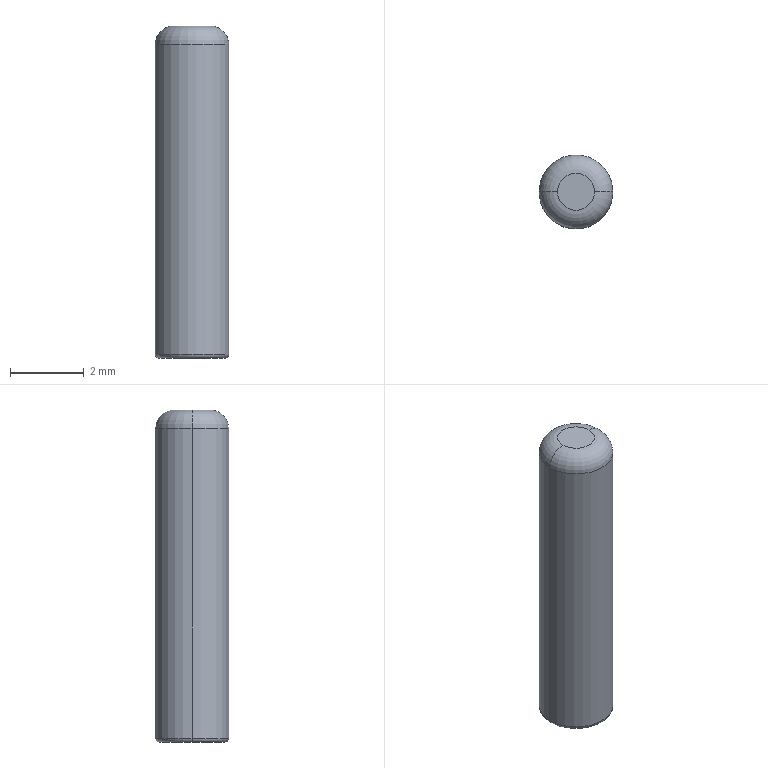Part | SolidWorks | features Fillet 2, Extrusion 1 | 1 solid | 8 faces | box 2 x 2 x 9 mm | volume 27.962 mm3 | torus 4 | cylinder 2 | plane 2 | commonest cylinder face diameters 2 x2
STEP:
#1=CARTESIAN_POINT('',(-0.9,0.,0.));
#2=VERTEX_POINT('',#1);
#3=CARTESIAN_POINT('',(0.9,0.,0.));
#4=VERTEX_POINT('',#3);
#5=CARTESIAN_POINT('',(0.,0.,0.));
#6=DIRECTION('',(0.,0.,-1.));
#7=DIRECTION('',(1.,0.,0.));
#8=AXIS2_PLACEMENT_3D('',#5,#6,#7);
#9=CIRCLE('',#8,0.9);
#10=EDGE_CURVE('',#2,#4,#9,.T.);
#11=ORIENTED_EDGE('',*,*,#10,.F.);
#12=CARTESIAN_POINT('',(-1.,0.,0.1));
#13=VERTEX_POINT('',#12);
#14=CARTESIAN_POINT('',(-0.9,0.,0.1));
#15=DIRECTION('',(0.,1.,0.));
#16=DIRECTION('',(-1.,0.,0.));
#17=AXIS2_PLACEMENT_3D('',#14,#15,#16);
#18=CIRCLE('',#17,0.1);
#19=EDGE_CURVE('',#2,#13,#18,.T.);
#20=ORIENTED_EDGE('',*,*,#19,.T.);
#21=CARTESIAN_POINT('',(1.,0.,0.1));
#22=VERTEX_POINT('',#21);
#23=CARTESIAN_POINT('',(0.,0.,0.1));
#24=DIRECTION('',(0.,0.,1.));
#25=DIRECTION('',(1.,0.,0.));
#26=AXIS2_PLACEMENT_3D('',#23,#24,#25);
#27=CIRCLE('',#26,1.);
#28=EDGE_CURVE('',#22,#13,#27,.T.);
#29=ORIENTED_EDGE('',*,*,#28,.F.);
#30=CARTESIAN_POINT('',(0.9,0.,0.1));
#31=DIRECTION('',(0.,-1.,0.));
#32=DIRECTION('',(0.,0.,-1.));
#33=AXIS2_PLACEMENT_3D('',#30,#31,#32);
#34=CIRCLE('',#33,0.1);
#35=EDGE_CURVE('',#4,#22,#34,.T.);
#36=ORIENTED_EDGE('',*,*,#35,.F.);
#37=EDGE_LOOP('',(#11,#20,#29,#36));
#38=FACE_OUTER_BOUND('',#37,.T.);
#39=CARTESIAN_POINT('',(0.,0.,0.1));
#40=DIRECTION('',(0.,0.,1.));
#41=DIRECTION('',(1.,0.,0.));
#42=AXIS2_PLACEMENT_3D('',#39,#40,#41);
#43=TOROIDAL_SURFACE('',#42,0.9,0.1);
#44=ADVANCED_FACE('',(#38),#43,.T.);
#45=CARTESIAN_POINT('',(-1.,0.,8.5));
#46=VERTEX_POINT('',#45);
#47=CARTESIAN_POINT('',(1.,0.,8.5));
#48=VERTEX_POINT('',#47);
#49=CARTESIAN_POINT('',(0.,0.,8.5));
#50=DIRECTION('',(0.,0.,-1.));
#51=DIRECTION('',(1.,0.,0.));
#52=AXIS2_PLACEMENT_3D('',#49,#50,#51);
#53=CIRCLE('',#52,1.);
#54=EDGE_CURVE('',#46,#48,#53,.T.);
#55=ORIENTED_EDGE('',*,*,#54,.F.);
#56=CARTESIAN_POINT('',(-0.5,0.,9.));
#57=VERTEX_POINT('',#56);
#58=CARTESIAN_POINT('',(-0.5,0.,8.5));
#59=DIRECTION('',(0.,1.,0.));
#60=DIRECTION('',(-1.,0.,0.));
#61=AXIS2_PLACEMENT_3D('',#58,#59,#60);
#62=CIRCLE('',#61,0.5);
#63=EDGE_CURVE('',#46,#57,#62,.T.);
#64=ORIENTED_EDGE('',*,*,#63,.T.);
#65=CARTESIAN_POINT('',(0.5,0.,9.));
#66=VERTEX_POINT('',#65);
#67=CARTESIAN_POINT('',(0.,0.,9.));
#68=DIRECTION('',(0.,0.,1.));
#69=DIRECTION('',(1.,0.,0.));
#70=AXIS2_PLACEMENT_3D('',#67,#68,#69);
#71=CIRCLE('',#70,0.5);
#72=EDGE_CURVE('',#66,#57,#71,.T.);
#73=ORIENTED_EDGE('',*,*,#72,.F.);
#74=CARTESIAN_POINT('',(0.5,0.,8.5));
#75=DIRECTION('',(0.,-1.,0.));
#76=DIRECTION('',(0.,0.,-1.));
#77=AXIS2_PLACEMENT_3D('',#74,#75,#76);
#78=CIRCLE('',#77,0.5);
#79=EDGE_CURVE('',#48,#66,#78,.T.);
#80=ORIENTED_EDGE('',*,*,#79,.F.);
#81=EDGE_LOOP('',(#55,#64,#73,#80));
#82=FACE_OUTER_BOUND('',#81,.T.);
#83=CARTESIAN_POINT('',(0.,0.,8.5));
#84=DIRECTION('',(0.,0.,1.));
#85=DIRECTION('',(1.,0.,0.));
#86=AXIS2_PLACEMENT_3D('',#83,#84,#85);
#87=TOROIDAL_SURFACE('',#86,0.5,0.5);
#88=ADVANCED_FACE('',(#82),#87,.T.);
#89=ORIENTED_EDGE('',*,*,#54,.T.);
#90=CARTESIAN_POINT('',(1.,0.,9.));
#91=DIRECTION('',(0.,0.,-1.));
#92=VECTOR('',#91,1000.);
#93=LINE('',#90,#92);
#94=EDGE_CURVE('',#48,#22,#93,.T.);
#95=ORIENTED_EDGE('',*,*,#94,.T.);
#96=ORIENTED_EDGE('',*,*,#28,.T.);
#97=CARTESIAN_POINT('',(-1.,0.,9.));
#98=DIRECTION('',(0.,0.,-1.));
#99=VECTOR('',#98,1000.);
#100=LINE('',#97,#99);
#101=EDGE_CURVE('',#46,#13,#100,.T.);
#102=ORIENTED_EDGE('',*,*,#101,.F.);
#103=EDGE_LOOP('',(#89,#95,#96,#102));
#104=FACE_OUTER_BOUND('',#103,.T.);
#105=CARTESIAN_POINT('',(0.,0.,9.));
#106=DIRECTION('',(0.,0.,-1.));
#107=DIRECTION('',(-1.,0.,0.));
#108=AXIS2_PLACEMENT_3D('',#105,#106,#107);
#109=CYLINDRICAL_SURFACE('',#108,1.);
#110=ADVANCED_FACE('',(#104),#109,.T.);
#111=ORIENTED_EDGE('',*,*,#94,.F.);
#112=CARTESIAN_POINT('',(0.,0.,8.5));
#113=DIRECTION('',(0.,0.,-1.));
#114=DIRECTION('',(1.,0.,0.));
#115=AXIS2_PLACEMENT_3D('',#112,#113,#114);
#116=CIRCLE('',#115,1.);
#117=EDGE_CURVE('',#48,#46,#116,.T.);
#118=ORIENTED_EDGE('',*,*,#117,.T.);
#119=ORIENTED_EDGE('',*,*,#101,.T.);
#120=CARTESIAN_POINT('',(0.,0.,0.1));
#121=DIRECTION('',(0.,0.,1.));
#122=DIRECTION('',(1.,0.,0.));
#123=AXIS2_PLACEMENT_3D('',#120,#121,#122);
#124=CIRCLE('',#123,1.);
#125=EDGE_CURVE('',#13,#22,#124,.T.);
#126=ORIENTED_EDGE('',*,*,#125,.T.);
#127=EDGE_LOOP('',(#111,#118,#119,#126));
#128=FACE_OUTER_BOUND('',#127,.T.);
#129=CARTESIAN_POINT('',(0.,0.,9.));
#130=DIRECTION('',(0.,0.,-1.));
#131=DIRECTION('',(-1.,0.,0.));
#132=AXIS2_PLACEMENT_3D('',#129,#130,#131);
#133=CYLINDRICAL_SURFACE('',#132,1.);
#134=ADVANCED_FACE('',(#128),#133,.T.);
#135=ORIENTED_EDGE('',*,*,#72,.T.);
#136=CARTESIAN_POINT('',(0.,0.,9.));
#137=DIRECTION('',(0.,0.,1.));
#138=DIRECTION('',(1.,0.,0.));
#139=AXIS2_PLACEMENT_3D('',#136,#137,#138);
#140=CIRCLE('',#139,0.5);
#141=EDGE_CURVE('',#57,#66,#140,.T.);
#142=ORIENTED_EDGE('',*,*,#141,.T.);
#143=EDGE_LOOP('',(#135,#142));
#144=FACE_OUTER_BOUND('',#143,.T.);
#145=CARTESIAN_POINT('',(0.,0.,9.));
#146=DIRECTION('',(0.,0.,1.));
#147=DIRECTION('',(1.,0.,0.));
#148=AXIS2_PLACEMENT_3D('',#145,#146,#147);
#149=PLANE('',#148);
#150=ADVANCED_FACE('',(#144),#149,.T.);
#151=CARTESIAN_POINT('',(0.,0.,0.));
#152=DIRECTION('',(0.,0.,-1.));
#153=DIRECTION('',(1.,0.,0.));
#154=AXIS2_PLACEMENT_3D('',#151,#152,#153);
#155=CIRCLE('',#154,0.9);
#156=EDGE_CURVE('',#4,#2,#155,.T.);
#157=ORIENTED_EDGE('',*,*,#156,.T.);
#158=ORIENTED_EDGE('',*,*,#10,.T.);
#159=EDGE_LOOP('',(#157,#158));
#160=FACE_OUTER_BOUND('',#159,.T.);
#161=CARTESIAN_POINT('',(0.,0.,0.));
#162=DIRECTION('',(0.,0.,1.));
#163=DIRECTION('',(1.,0.,0.));
#164=AXIS2_PLACEMENT_3D('',#161,#162,#163);
#165=PLANE('',#164);
#166=ADVANCED_FACE('',(#160),#165,.F.);
#167=ORIENTED_EDGE('',*,*,#63,.F.);
#168=ORIENTED_EDGE('',*,*,#117,.F.);
#169=ORIENTED_EDGE('',*,*,#79,.T.);
#170=ORIENTED_EDGE('',*,*,#141,.F.);
#171=EDGE_LOOP('',(#167,#168,#169,#170));
#172=FACE_OUTER_BOUND('',#171,.T.);
#173=CARTESIAN_POINT('',(0.,0.,8.5));
#174=DIRECTION('',(0.,0.,1.));
#175=DIRECTION('',(1.,0.,0.));
#176=AXIS2_PLACEMENT_3D('',#173,#174,#175);
#177=TOROIDAL_SURFACE('',#176,0.5,0.5);
#178=ADVANCED_FACE('',(#172),#177,.T.);
#179=ORIENTED_EDGE('',*,*,#19,.F.);
#180=ORIENTED_EDGE('',*,*,#156,.F.);
#181=ORIENTED_EDGE('',*,*,#35,.T.);
#182=ORIENTED_EDGE('',*,*,#125,.F.);
#183=EDGE_LOOP('',(#179,#180,#181,#182));
#184=FACE_OUTER_BOUND('',#183,.T.);
#185=CARTESIAN_POINT('',(0.,0.,0.1));
#186=DIRECTION('',(0.,0.,1.));
#187=DIRECTION('',(1.,0.,0.));
#188=AXIS2_PLACEMENT_3D('',#185,#186,#187);
#189=TOROIDAL_SURFACE('',#188,0.9,0.1);
#190=ADVANCED_FACE('',(#184),#189,.T.);
#191=CLOSED_SHELL('',(#44,#88,#110,#134,#150,#166,#178,#190));
#192=MANIFOLD_SOLID_BREP('',#191);
#193=CARTESIAN_POINT('',(0.,0.,0.));
#194=DIRECTION('',(0.,0.,1.));
#195=DIRECTION('',(1.,0.,0.));
#196=AXIS2_PLACEMENT_3D('',#193,#194,#195);
#197=(LENGTH_UNIT()NAMED_UNIT(*)SI_UNIT(.MILLI.,.METRE.));
#198=UNCERTAINTY_MEASURE_WITH_UNIT(LENGTH_MEASURE(0.00001),#197,'','');
#199=(NAMED_UNIT(*)PLANE_ANGLE_UNIT()SI_UNIT($,.RADIAN.));
#200=(NAMED_UNIT(*)SI_UNIT($,.STERADIAN.)SOLID_ANGLE_UNIT());
#201=(GEOMETRIC_REPRESENTATION_CONTEXT(3)GLOBAL_UNCERTAINTY_ASSIGNED_CONTEXT((#198))GLOBAL_UNIT_ASSIGNED_CONTEXT((#197,#199,#200))REPRESENTATION_CONTEXT('',''));
#202=ADVANCED_BREP_SHAPE_REPRESENTATION('',(#192,#196),#201);